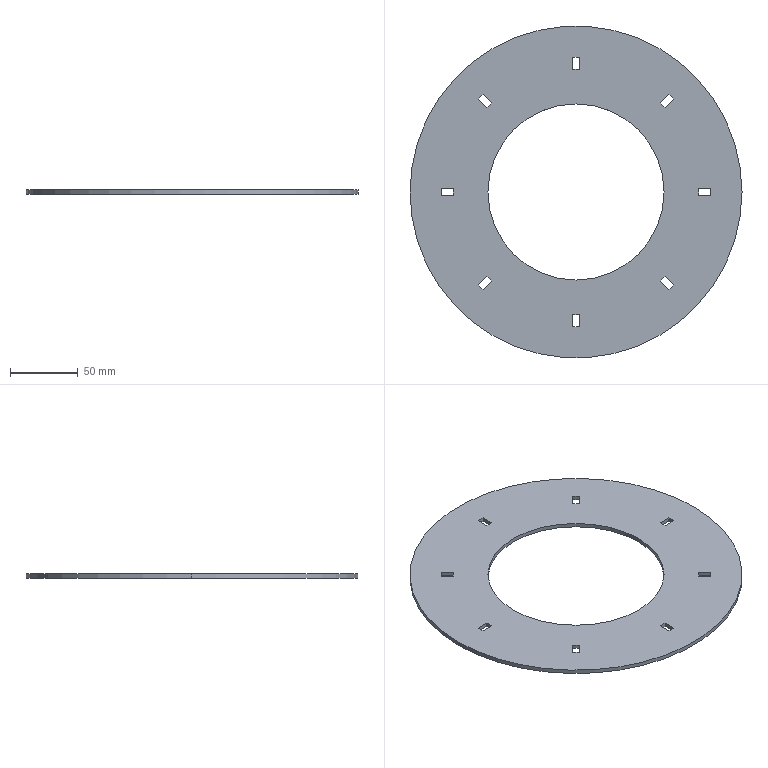Part | SolidWorks | features CirPattern 1, Extrusion 1, ICE 1 | 1 solid | 38 faces | box 245 x 245 x 3 mm | volume 100531 mm3 | plane 34 | cylinder 4 | commonest cylinder face diameters 130 x2 245 x2
STEP:
#1=CARTESIAN_POINT('',(-65.,0.,3.));
#2=VERTEX_POINT('',#1);
#3=CARTESIAN_POINT('',(65.,0.,3.));
#4=VERTEX_POINT('',#3);
#5=CARTESIAN_POINT('',(0.,0.,3.));
#6=DIRECTION('',(0.,0.,1.));
#7=DIRECTION('',(1.,0.,0.));
#8=AXIS2_PLACEMENT_3D('',#5,#6,#7);
#9=CIRCLE('',#8,65.);
#10=EDGE_CURVE('',#2,#4,#9,.T.);
#11=ORIENTED_EDGE('',*,*,#10,.T.);
#12=CARTESIAN_POINT('',(65.,0.,0.));
#13=VERTEX_POINT('',#12);
#14=CARTESIAN_POINT('',(65.,0.,3.));
#15=DIRECTION('',(0.,0.,-1.));
#16=VECTOR('',#15,1000.);
#17=LINE('',#14,#16);
#18=EDGE_CURVE('',#4,#13,#17,.T.);
#19=ORIENTED_EDGE('',*,*,#18,.T.);
#20=CARTESIAN_POINT('',(-65.,0.,0.));
#21=VERTEX_POINT('',#20);
#22=CARTESIAN_POINT('',(0.,0.,0.));
#23=DIRECTION('',(0.,0.,1.));
#24=DIRECTION('',(1.,0.,0.));
#25=AXIS2_PLACEMENT_3D('',#22,#23,#24);
#26=CIRCLE('',#25,65.);
#27=EDGE_CURVE('',#21,#13,#26,.T.);
#28=ORIENTED_EDGE('',*,*,#27,.F.);
#29=CARTESIAN_POINT('',(-65.,0.,3.));
#30=DIRECTION('',(0.,0.,-1.));
#31=VECTOR('',#30,1000.);
#32=LINE('',#29,#31);
#33=EDGE_CURVE('',#2,#21,#32,.T.);
#34=ORIENTED_EDGE('',*,*,#33,.F.);
#35=EDGE_LOOP('',(#11,#19,#28,#34));
#36=FACE_OUTER_BOUND('',#35,.T.);
#37=CARTESIAN_POINT('',(0.,0.,3.));
#38=DIRECTION('',(0.,0.,-1.));
#39=DIRECTION('',(-1.,0.,0.));
#40=AXIS2_PLACEMENT_3D('',#37,#38,#39);
#41=CYLINDRICAL_SURFACE('',#40,65.);
#42=ADVANCED_FACE('',(#36),#41,.F.);
#43=CARTESIAN_POINT('',(122.5,0.,3.));
#44=VERTEX_POINT('',#43);
#45=CARTESIAN_POINT('',(-122.5,0.,3.));
#46=VERTEX_POINT('',#45);
#47=CARTESIAN_POINT('',(0.,0.,3.));
#48=DIRECTION('',(0.,0.,1.));
#49=DIRECTION('',(1.,0.,0.));
#50=AXIS2_PLACEMENT_3D('',#47,#48,#49);
#51=CIRCLE('',#50,122.5);
#52=EDGE_CURVE('',#44,#46,#51,.T.);
#53=ORIENTED_EDGE('',*,*,#52,.F.);
#54=CARTESIAN_POINT('',(122.5,0.,0.));
#55=VERTEX_POINT('',#54);
#56=CARTESIAN_POINT('',(122.5,0.,3.));
#57=DIRECTION('',(0.,0.,-1.));
#58=VECTOR('',#57,1000.);
#59=LINE('',#56,#58);
#60=EDGE_CURVE('',#44,#55,#59,.T.);
#61=ORIENTED_EDGE('',*,*,#60,.T.);
#62=CARTESIAN_POINT('',(-122.5,0.,0.));
#63=VERTEX_POINT('',#62);
#64=CARTESIAN_POINT('',(0.,0.,0.));
#65=DIRECTION('',(0.,0.,1.));
#66=DIRECTION('',(1.,0.,0.));
#67=AXIS2_PLACEMENT_3D('',#64,#65,#66);
#68=CIRCLE('',#67,122.5);
#69=EDGE_CURVE('',#55,#63,#68,.T.);
#70=ORIENTED_EDGE('',*,*,#69,.T.);
#71=CARTESIAN_POINT('',(-122.5,0.,3.));
#72=DIRECTION('',(0.,0.,-1.));
#73=VECTOR('',#72,1000.);
#74=LINE('',#71,#73);
#75=EDGE_CURVE('',#46,#63,#74,.T.);
#76=ORIENTED_EDGE('',*,*,#75,.F.);
#77=EDGE_LOOP('',(#53,#61,#70,#76));
#78=FACE_OUTER_BOUND('',#77,.T.);
#79=CARTESIAN_POINT('',(0.,0.,3.));
#80=DIRECTION('',(0.,0.,-1.));
#81=DIRECTION('',(-1.,0.,0.));
#82=AXIS2_PLACEMENT_3D('',#79,#80,#81);
#83=CYLINDRICAL_SURFACE('',#82,122.5);
#84=ADVANCED_FACE('',(#78),#83,.T.);
#85=CARTESIAN_POINT('',(99.5,2.5,3.));
#86=VERTEX_POINT('',#85);
#87=CARTESIAN_POINT('',(90.5,2.5,3.));
#88=VERTEX_POINT('',#87);
#89=CARTESIAN_POINT('',(90.5,2.5,3.));
#90=DIRECTION('',(-1.,0.,0.));
#91=VECTOR('',#90,1000.);
#92=LINE('',#89,#91);
#93=EDGE_CURVE('',#86,#88,#92,.T.);
#94=ORIENTED_EDGE('',*,*,#93,.F.);
#95=CARTESIAN_POINT('',(99.5,-2.5,3.));
#96=VERTEX_POINT('',#95);
#97=CARTESIAN_POINT('',(99.5,-2.5,3.));
#98=DIRECTION('',(0.,1.,0.));
#99=VECTOR('',#98,1000.);
#100=LINE('',#97,#99);
#101=EDGE_CURVE('',#96,#86,#100,.T.);
#102=ORIENTED_EDGE('',*,*,#101,.F.);
#103=CARTESIAN_POINT('',(90.5,-2.5,3.));
#104=VERTEX_POINT('',#103);
#105=CARTESIAN_POINT('',(90.5,-2.5,3.));
#106=DIRECTION('',(1.,0.,0.));
#107=VECTOR('',#106,1000.);
#108=LINE('',#105,#107);
#109=EDGE_CURVE('',#104,#96,#108,.T.);
#110=ORIENTED_EDGE('',*,*,#109,.F.);
#111=CARTESIAN_POINT('',(90.5,-2.5,3.));
#112=DIRECTION('',(0.,-1.,0.));
#113=VECTOR('',#112,1000.);
#114=LINE('',#111,#113);
#115=EDGE_CURVE('',#88,#104,#114,.T.);
#116=ORIENTED_EDGE('',*,*,#115,.F.);
#117=EDGE_LOOP('',(#94,#102,#110,#116));
#118=FACE_BOUND('',#117,.T.);
#119=CARTESIAN_POINT('',(72.125,-68.589,3.));
#120=VERTEX_POINT('',#119);
#121=CARTESIAN_POINT('',(65.761,-62.225,3.));
#122=VERTEX_POINT('',#121);
#123=CARTESIAN_POINT('',(65.761,-62.225,3.));
#124=DIRECTION('',(-0.7071,0.7071,0.));
#125=VECTOR('',#124,1000.);
#126=LINE('',#123,#125);
#127=EDGE_CURVE('',#120,#122,#126,.T.);
#128=ORIENTED_EDGE('',*,*,#127,.F.);
#129=CARTESIAN_POINT('',(68.589,-72.125,3.));
#130=VERTEX_POINT('',#129);
#131=CARTESIAN_POINT('',(68.589,-72.125,3.));
#132=DIRECTION('',(0.7071,0.7071,0.));
#133=VECTOR('',#132,1000.);
#134=LINE('',#131,#133);
#135=EDGE_CURVE('',#130,#120,#134,.T.);
#136=ORIENTED_EDGE('',*,*,#135,.F.);
#137=CARTESIAN_POINT('',(62.225,-65.761,3.));
#138=VERTEX_POINT('',#137);
#139=CARTESIAN_POINT('',(62.225,-65.761,3.));
#140=DIRECTION('',(0.7071,-0.7071,0.));
#141=VECTOR('',#140,1000.);
#142=LINE('',#139,#141);
#143=EDGE_CURVE('',#138,#130,#142,.T.);
#144=ORIENTED_EDGE('',*,*,#143,.F.);
#145=CARTESIAN_POINT('',(62.225,-65.761,3.));
#146=DIRECTION('',(-0.7071,-0.7071,0.));
#147=VECTOR('',#146,1000.);
#148=LINE('',#145,#147);
#149=EDGE_CURVE('',#122,#138,#148,.T.);
#150=ORIENTED_EDGE('',*,*,#149,.F.);
#151=EDGE_LOOP('',(#128,#136,#144,#150));
#152=FACE_BOUND('',#151,.T.);
#153=CARTESIAN_POINT('',(2.5,-99.5,3.));
#154=VERTEX_POINT('',#153);
#155=CARTESIAN_POINT('',(2.5,-90.5,3.));
#156=VERTEX_POINT('',#155);
#157=CARTESIAN_POINT('',(2.5,-90.5,3.));
#158=DIRECTION('',(0.,1.,0.));
#159=VECTOR('',#158,1000.);
#160=LINE('',#157,#159);
#161=EDGE_CURVE('',#154,#156,#160,.T.);
#162=ORIENTED_EDGE('',*,*,#161,.F.);
#163=CARTESIAN_POINT('',(-2.5,-99.5,3.));
#164=VERTEX_POINT('',#163);
#165=CARTESIAN_POINT('',(-2.5,-99.5,3.));
#166=DIRECTION('',(1.,0.,0.));
#167=VECTOR('',#166,1000.);
#168=LINE('',#165,#167);
#169=EDGE_CURVE('',#164,#154,#168,.T.);
#170=ORIENTED_EDGE('',*,*,#169,.F.);
#171=CARTESIAN_POINT('',(-2.5,-90.5,3.));
#172=VERTEX_POINT('',#171);
#173=CARTESIAN_POINT('',(-2.5,-90.5,3.));
#174=DIRECTION('',(0.,-1.,0.));
#175=VECTOR('',#174,1000.);
#176=LINE('',#173,#175);
#177=EDGE_CURVE('',#172,#164,#176,.T.);
#178=ORIENTED_EDGE('',*,*,#177,.F.);
#179=CARTESIAN_POINT('',(-2.5,-90.5,3.));
#180=DIRECTION('',(-1.,0.,0.));
#181=VECTOR('',#180,1000.);
#182=LINE('',#179,#181);
#183=EDGE_CURVE('',#156,#172,#182,.T.);
#184=ORIENTED_EDGE('',*,*,#183,.F.);
#185=EDGE_LOOP('',(#162,#170,#178,#184));
#186=FACE_BOUND('',#185,.T.);
#187=CARTESIAN_POINT('',(-68.589,-72.125,3.));
#188=VERTEX_POINT('',#187);
#189=CARTESIAN_POINT('',(-62.225,-65.761,3.));
#190=VERTEX_POINT('',#189);
#191=CARTESIAN_POINT('',(-62.225,-65.761,3.));
#192=DIRECTION('',(0.7071,0.7071,0.));
#193=VECTOR('',#192,1000.);
#194=LINE('',#191,#193);
#195=EDGE_CURVE('',#188,#190,#194,.T.);
#196=ORIENTED_EDGE('',*,*,#195,.F.);
#197=CARTESIAN_POINT('',(-72.125,-68.589,3.));
#198=VERTEX_POINT('',#197);
#199=CARTESIAN_POINT('',(-72.125,-68.589,3.));
#200=DIRECTION('',(0.7071,-0.7071,0.));
#201=VECTOR('',#200,1000.);
#202=LINE('',#199,#201);
#203=EDGE_CURVE('',#198,#188,#202,.T.);
#204=ORIENTED_EDGE('',*,*,#203,.F.);
#205=CARTESIAN_POINT('',(-65.761,-62.225,3.));
#206=VERTEX_POINT('',#205);
#207=CARTESIAN_POINT('',(-65.761,-62.225,3.));
#208=DIRECTION('',(-0.7071,-0.7071,0.));
#209=VECTOR('',#208,1000.);
#210=LINE('',#207,#209);
#211=EDGE_CURVE('',#206,#198,#210,.T.);
#212=ORIENTED_EDGE('',*,*,#211,.F.);
#213=CARTESIAN_POINT('',(-65.761,-62.225,3.));
#214=DIRECTION('',(-0.7071,0.7071,0.));
#215=VECTOR('',#214,1000.);
#216=LINE('',#213,#215);
#217=EDGE_CURVE('',#190,#206,#216,.T.);
#218=ORIENTED_EDGE('',*,*,#217,.F.);
#219=EDGE_LOOP('',(#196,#204,#212,#218));
#220=FACE_BOUND('',#219,.T.);
#221=CARTESIAN_POINT('',(-99.5,-2.5,3.));
#222=VERTEX_POINT('',#221);
#223=CARTESIAN_POINT('',(-90.5,-2.5,3.));
#224=VERTEX_POINT('',#223);
#225=CARTESIAN_POINT('',(-90.5,-2.5,3.));
#226=DIRECTION('',(1.,0.,0.));
#227=VECTOR('',#226,1000.);
#228=LINE('',#225,#227);
#229=EDGE_CURVE('',#222,#224,#228,.T.);
#230=ORIENTED_EDGE('',*,*,#229,.F.);
#231=CARTESIAN_POINT('',(-99.5,2.5,3.));
#232=VERTEX_POINT('',#231);
#233=CARTESIAN_POINT('',(-99.5,2.5,3.));
#234=DIRECTION('',(0.,-1.,0.));
#235=VECTOR('',#234,1000.);
#236=LINE('',#233,#235);
#237=EDGE_CURVE('',#232,#222,#236,.T.);
#238=ORIENTED_EDGE('',*,*,#237,.F.);
#239=CARTESIAN_POINT('',(-90.5,2.5,3.));
#240=VERTEX_POINT('',#239);
#241=CARTESIAN_POINT('',(-90.5,2.5,3.));
#242=DIRECTION('',(-1.,0.,0.));
#243=VECTOR('',#242,1000.);
#244=LINE('',#241,#243);
#245=EDGE_CURVE('',#240,#232,#244,.T.);
#246=ORIENTED_EDGE('',*,*,#245,.F.);
#247=CARTESIAN_POINT('',(-90.5,2.5,3.));
#248=DIRECTION('',(0.,1.,0.));
#249=VECTOR('',#248,1000.);
#250=LINE('',#247,#249);
#251=EDGE_CURVE('',#224,#240,#250,.T.);
#252=ORIENTED_EDGE('',*,*,#251,.F.);
#253=EDGE_LOOP('',(#230,#238,#246,#252));
#254=FACE_BOUND('',#253,.T.);
#255=CARTESIAN_POINT('',(-72.125,68.589,3.));
#256=VERTEX_POINT('',#255);
#257=CARTESIAN_POINT('',(-65.761,62.225,3.));
#258=VERTEX_POINT('',#257);
#259=CARTESIAN_POINT('',(-65.761,62.225,3.));
#260=DIRECTION('',(0.7071,-0.7071,0.));
#261=VECTOR('',#260,1000.);
#262=LINE('',#259,#261);
#263=EDGE_CURVE('',#256,#258,#262,.T.);
#264=ORIENTED_EDGE('',*,*,#263,.F.);
#265=CARTESIAN_POINT('',(-68.589,72.125,3.));
#266=VERTEX_POINT('',#265);
#267=CARTESIAN_POINT('',(-68.589,72.125,3.));
#268=DIRECTION('',(-0.7071,-0.7071,0.));
#269=VECTOR('',#268,1000.);
#270=LINE('',#267,#269);
#271=EDGE_CURVE('',#266,#256,#270,.T.);
#272=ORIENTED_EDGE('',*,*,#271,.F.);
#273=CARTESIAN_POINT('',(-62.225,65.761,3.));
#274=VERTEX_POINT('',#273);
#275=CARTESIAN_POINT('',(-62.225,65.761,3.));
#276=DIRECTION('',(-0.7071,0.7071,0.));
#277=VECTOR('',#276,1000.);
#278=LINE('',#275,#277);
#279=EDGE_CURVE('',#274,#266,#278,.T.);
#280=ORIENTED_EDGE('',*,*,#279,.F.);
#281=CARTESIAN_POINT('',(-62.225,65.761,3.));
#282=DIRECTION('',(0.7071,0.7071,0.));
#283=VECTOR('',#282,1000.);
#284=LINE('',#281,#283);
#285=EDGE_CURVE('',#258,#274,#284,.T.);
#286=ORIENTED_EDGE('',*,*,#285,.F.);
#287=EDGE_LOOP('',(#264,#272,#280,#286));
#288=FACE_BOUND('',#287,.T.);
#289=CARTESIAN_POINT('',(68.589,72.125,3.));
#290=VERTEX_POINT('',#289);
#291=CARTESIAN_POINT('',(62.225,65.761,3.));
#292=VERTEX_POINT('',#291);
#293=CARTESIAN_POINT('',(62.225,65.761,3.));
#294=DIRECTION('',(-0.7071,-0.7071,0.));
#295=VECTOR('',#294,1000.);
#296=LINE('',#293,#295);
#297=EDGE_CURVE('',#290,#292,#296,.T.);
#298=ORIENTED_EDGE('',*,*,#297,.F.);
#299=CARTESIAN_POINT('',(72.125,68.589,3.));
#300=VERTEX_POINT('',#299);
#301=CARTESIAN_POINT('',(72.125,68.589,3.));
#302=DIRECTION('',(-0.7071,0.7071,0.));
#303=VECTOR('',#302,1000.);
#304=LINE('',#301,#303);
#305=EDGE_CURVE('',#300,#290,#304,.T.);
#306=ORIENTED_EDGE('',*,*,#305,.F.);
#307=CARTESIAN_POINT('',(65.761,62.225,3.));
#308=VERTEX_POINT('',#307);
#309=CARTESIAN_POINT('',(65.761,62.225,3.));
#310=DIRECTION('',(0.7071,0.7071,0.));
#311=VECTOR('',#310,1000.);
#312=LINE('',#309,#311);
#313=EDGE_CURVE('',#308,#300,#312,.T.);
#314=ORIENTED_EDGE('',*,*,#313,.F.);
#315=CARTESIAN_POINT('',(65.761,62.225,3.));
#316=DIRECTION('',(0.7071,-0.7071,0.));
#317=VECTOR('',#316,1000.);
#318=LINE('',#315,#317);
#319=EDGE_CURVE('',#292,#308,#318,.T.);
#320=ORIENTED_EDGE('',*,*,#319,.F.);
#321=EDGE_LOOP('',(#298,#306,#314,#320));
#322=FACE_BOUND('',#321,.T.);
#323=CARTESIAN_POINT('',(-2.5,99.5,3.));
#324=VERTEX_POINT('',#323);
#325=CARTESIAN_POINT('',(-2.5,90.5,3.));
#326=VERTEX_POINT('',#325);
#327=CARTESIAN_POINT('',(-2.5,90.5,3.));
#328=DIRECTION('',(0.,-1.,0.));
#329=VECTOR('',#328,1000.);
#330=LINE('',#327,#329);
#331=EDGE_CURVE('',#324,#326,#330,.T.);
#332=ORIENTED_EDGE('',*,*,#331,.F.);
#333=CARTESIAN_POINT('',(2.5,99.5,3.));
#334=VERTEX_POINT('',#333);
#335=CARTESIAN_POINT('',(2.5,99.5,3.));
#336=DIRECTION('',(-1.,0.,0.));
#337=VECTOR('',#336,1000.);
#338=LINE('',#335,#337);
#339=EDGE_CURVE('',#334,#324,#338,.T.);
#340=ORIENTED_EDGE('',*,*,#339,.F.);
#341=CARTESIAN_POINT('',(2.5,90.5,3.));
#342=VERTEX_POINT('',#341);
#343=CARTESIAN_POINT('',(2.5,90.5,3.));
#344=DIRECTION('',(0.,1.,0.));
#345=VECTOR('',#344,1000.);
#346=LINE('',#343,#345);
#347=EDGE_CURVE('',#342,#334,#346,.T.);
#348=ORIENTED_EDGE('',*,*,#347,.F.);
#349=CARTESIAN_POINT('',(2.5,90.5,3.));
#350=DIRECTION('',(1.,0.,0.));
#351=VECTOR('',#350,1000.);
#352=LINE('',#349,#351);
#353=EDGE_CURVE('',#326,#342,#352,.T.);
#354=ORIENTED_EDGE('',*,*,#353,.F.);
#355=EDGE_LOOP('',(#332,#340,#348,#354));
#356=FACE_BOUND('',#355,.T.);
#357=CARTESIAN_POINT('',(0.,0.,3.));
#358=DIRECTION('',(0.,0.,1.));
#359=DIRECTION('',(1.,0.,0.));
#360=AXIS2_PLACEMENT_3D('',#357,#358,#359);
#361=CIRCLE('',#360,122.5);
#362=EDGE_CURVE('',#46,#44,#361,.T.);
#363=ORIENTED_EDGE('',*,*,#362,.T.);
#364=ORIENTED_EDGE('',*,*,#52,.T.);
#365=EDGE_LOOP('',(#363,#364));
#366=FACE_OUTER_BOUND('',#365,.T.);
#367=ORIENTED_EDGE('',*,*,#10,.F.);
#368=CARTESIAN_POINT('',(0.,0.,3.));
#369=DIRECTION('',(0.,0.,1.));
#370=DIRECTION('',(1.,0.,0.));
#371=AXIS2_PLACEMENT_3D('',#368,#369,#370);
#372=CIRCLE('',#371,65.);
#373=EDGE_CURVE('',#4,#2,#372,.T.);
#374=ORIENTED_EDGE('',*,*,#373,.F.);
#375=EDGE_LOOP('',(#367,#374));
#376=FACE_BOUND('',#375,.T.);
#377=CARTESIAN_POINT('',(0.,0.,3.));
#378=DIRECTION('',(0.,0.,1.));
#379=DIRECTION('',(1.,0.,0.));
#380=AXIS2_PLACEMENT_3D('',#377,#378,#379);
#381=PLANE('',#380);
#382=ADVANCED_FACE('',(#118,#152,#186,#220,#254,#288,#322,#356,#366,#376),#381,.T.);
#383=CARTESIAN_POINT('',(99.5,-2.5,0.));
#384=VERTEX_POINT('',#383);
#385=CARTESIAN_POINT('',(99.5,2.5,0.));
#386=VERTEX_POINT('',#385);
#387=CARTESIAN_POINT('',(99.5,0.,0.));
#388=DIRECTION('',(0.,1.,0.));
#389=VECTOR('',#388,1000.);
#390=LINE('',#387,#389);
#391=EDGE_CURVE('',#384,#386,#390,.T.);
#392=ORIENTED_EDGE('',*,*,#391,.T.);
#393=CARTESIAN_POINT('',(90.5,2.5,0.));
#394=VERTEX_POINT('',#393);
#395=CARTESIAN_POINT('',(0.,2.5,0.));
#396=DIRECTION('',(-1.,0.,0.));
#397=VECTOR('',#396,1000.);
#398=LINE('',#395,#397);
#399=EDGE_CURVE('',#386,#394,#398,.T.);
#400=ORIENTED_EDGE('',*,*,#399,.T.);
#401=CARTESIAN_POINT('',(90.5,-2.5,0.));
#402=VERTEX_POINT('',#401);
#403=CARTESIAN_POINT('',(90.5,0.,0.));
#404=DIRECTION('',(0.,-1.,0.));
#405=VECTOR('',#404,1000.);
#406=LINE('',#403,#405);
#407=EDGE_CURVE('',#394,#402,#406,.T.);
#408=ORIENTED_EDGE('',*,*,#407,.T.);
#409=CARTESIAN_POINT('',(0.,-2.5,0.));
#410=DIRECTION('',(1.,0.,0.));
#411=VECTOR('',#410,1000.);
#412=LINE('',#409,#411);
#413=EDGE_CURVE('',#402,#384,#412,.T.);
#414=ORIENTED_EDGE('',*,*,#413,.T.);
#415=EDGE_LOOP('',(#392,#400,#408,#414));
#416=FACE_BOUND('',#415,.T.);
#417=CARTESIAN_POINT('',(68.589,-72.125,0.));
#418=VERTEX_POINT('',#417);
#419=CARTESIAN_POINT('',(72.125,-68.589,0.));
#420=VERTEX_POINT('',#419);
#421=CARTESIAN_POINT('',(70.357,-70.357,0.));
#422=DIRECTION('',(0.7071,0.7071,0.));
#423=VECTOR('',#422,1000.);
#424=LINE('',#421,#423);
#425=EDGE_CURVE('',#418,#420,#424,.T.);
#426=ORIENTED_EDGE('',*,*,#425,.T.);
#427=CARTESIAN_POINT('',(65.761,-62.225,0.));
#428=VERTEX_POINT('',#427);
#429=CARTESIAN_POINT('',(1.768,1.768,0.));
#430=DIRECTION('',(-0.7071,0.7071,0.));
#431=VECTOR('',#430,1000.);
#432=LINE('',#429,#431);
#433=EDGE_CURVE('',#420,#428,#432,.T.);
#434=ORIENTED_EDGE('',*,*,#433,.T.);
#435=CARTESIAN_POINT('',(62.225,-65.761,0.));
#436=VERTEX_POINT('',#435);
#437=CARTESIAN_POINT('',(63.993,-63.993,0.));
#438=DIRECTION('',(-0.7071,-0.7071,0.));
#439=VECTOR('',#438,1000.);
#440=LINE('',#437,#439);
#441=EDGE_CURVE('',#428,#436,#440,.T.);
#442=ORIENTED_EDGE('',*,*,#441,.T.);
#443=CARTESIAN_POINT('',(-1.768,-1.768,0.));
#444=DIRECTION('',(0.7071,-0.7071,0.));
#445=VECTOR('',#444,1000.);
#446=LINE('',#443,#445);
#447=EDGE_CURVE('',#436,#418,#446,.T.);
#448=ORIENTED_EDGE('',*,*,#447,.T.);
#449=EDGE_LOOP('',(#426,#434,#442,#448));
#450=FACE_BOUND('',#449,.T.);
#451=CARTESIAN_POINT('',(-2.5,-99.5,0.));
#452=VERTEX_POINT('',#451);
#453=CARTESIAN_POINT('',(2.5,-99.5,0.));
#454=VERTEX_POINT('',#453);
#455=CARTESIAN_POINT('',(0.,-99.5,0.));
#456=DIRECTION('',(1.,0.,0.));
#457=VECTOR('',#456,1000.);
#458=LINE('',#455,#457);
#459=EDGE_CURVE('',#452,#454,#458,.T.);
#460=ORIENTED_EDGE('',*,*,#459,.T.);
#461=CARTESIAN_POINT('',(2.5,-90.5,0.));
#462=VERTEX_POINT('',#461);
#463=CARTESIAN_POINT('',(2.5,0.,0.));
#464=DIRECTION('',(0.,1.,0.));
#465=VECTOR('',#464,1000.);
#466=LINE('',#463,#465);
#467=EDGE_CURVE('',#454,#462,#466,.T.);
#468=ORIENTED_EDGE('',*,*,#467,.T.);
#469=CARTESIAN_POINT('',(-2.5,-90.5,0.));
#470=VERTEX_POINT('',#469);
#471=CARTESIAN_POINT('',(0.,-90.5,0.));
#472=DIRECTION('',(-1.,0.,0.));
#473=VECTOR('',#472,1000.);
#474=LINE('',#471,#473);
#475=EDGE_CURVE('',#462,#470,#474,.T.);
#476=ORIENTED_EDGE('',*,*,#475,.T.);
#477=CARTESIAN_POINT('',(-2.5,0.,0.));
#478=DIRECTION('',(0.,-1.,0.));
#479=VECTOR('',#478,1000.);
#480=LINE('',#477,#479);
#481=EDGE_CURVE('',#470,#452,#480,.T.);
#482=ORIENTED_EDGE('',*,*,#481,.T.);
#483=EDGE_LOOP('',(#460,#468,#476,#482));
#484=FACE_BOUND('',#483,.T.);
#485=CARTESIAN_POINT('',(-72.125,-68.589,0.));
#486=VERTEX_POINT('',#485);
#487=CARTESIAN_POINT('',(-68.589,-72.125,0.));
#488=VERTEX_POINT('',#487);
#489=CARTESIAN_POINT('',(-70.357,-70.357,0.));
#490=DIRECTION('',(0.7071,-0.7071,0.));
#491=VECTOR('',#490,1000.);
#492=LINE('',#489,#491);
#493=EDGE_CURVE('',#486,#488,#492,.T.);
#494=ORIENTED_EDGE('',*,*,#493,.T.);
#495=CARTESIAN_POINT('',(-62.225,-65.761,0.));
#496=VERTEX_POINT('',#495);
#497=CARTESIAN_POINT('',(1.768,-1.768,0.));
#498=DIRECTION('',(0.7071,0.7071,0.));
#499=VECTOR('',#498,1000.);
#500=LINE('',#497,#499);
#501=EDGE_CURVE('',#488,#496,#500,.T.);
#502=ORIENTED_EDGE('',*,*,#501,.T.);
#503=CARTESIAN_POINT('',(-65.761,-62.225,0.));
#504=VERTEX_POINT('',#503);
#505=CARTESIAN_POINT('',(-63.993,-63.993,0.));
#506=DIRECTION('',(-0.7071,0.7071,0.));
#507=VECTOR('',#506,1000.);
#508=LINE('',#505,#507);
#509=EDGE_CURVE('',#496,#504,#508,.T.);
#510=ORIENTED_EDGE('',*,*,#509,.T.);
#511=CARTESIAN_POINT('',(-1.768,1.768,0.));
#512=DIRECTION('',(-0.7071,-0.7071,0.));
#513=VECTOR('',#512,1000.);
#514=LINE('',#511,#513);
#515=EDGE_CURVE('',#504,#486,#514,.T.);
#516=ORIENTED_EDGE('',*,*,#515,.T.);
#517=EDGE_LOOP('',(#494,#502,#510,#516));
#518=FACE_BOUND('',#517,.T.);
#519=CARTESIAN_POINT('',(-99.5,2.5,0.));
#520=VERTEX_POINT('',#519);
#521=CARTESIAN_POINT('',(-99.5,-2.5,0.));
#522=VERTEX_POINT('',#521);
#523=CARTESIAN_POINT('',(-99.5,0.,0.));
#524=DIRECTION('',(0.,-1.,0.));
#525=VECTOR('',#524,1000.);
#526=LINE('',#523,#525);
#527=EDGE_CURVE('',#520,#522,#526,.T.);
#528=ORIENTED_EDGE('',*,*,#527,.T.);
#529=CARTESIAN_POINT('',(-90.5,-2.5,0.));
#530=VERTEX_POINT('',#529);
#531=CARTESIAN_POINT('',(0.,-2.5,0.));
#532=DIRECTION('',(1.,0.,0.));
#533=VECTOR('',#532,1000.);
#534=LINE('',#531,#533);
#535=EDGE_CURVE('',#522,#530,#534,.T.);
#536=ORIENTED_EDGE('',*,*,#535,.T.);
#537=CARTESIAN_POINT('',(-90.5,2.5,0.));
#538=VERTEX_POINT('',#537);
#539=CARTESIAN_POINT('',(-90.5,0.,0.));
#540=DIRECTION('',(0.,1.,0.));
#541=VECTOR('',#540,1000.);
#542=LINE('',#539,#541);
#543=EDGE_CURVE('',#530,#538,#542,.T.);
#544=ORIENTED_EDGE('',*,*,#543,.T.);
#545=CARTESIAN_POINT('',(0.,2.5,0.));
#546=DIRECTION('',(-1.,0.,0.));
#547=VECTOR('',#546,1000.);
#548=LINE('',#545,#547);
#549=EDGE_CURVE('',#538,#520,#548,.T.);
#550=ORIENTED_EDGE('',*,*,#549,.T.);
#551=EDGE_LOOP('',(#528,#536,#544,#550));
#552=FACE_BOUND('',#551,.T.);
#553=CARTESIAN_POINT('',(-68.589,72.125,0.));
#554=VERTEX_POINT('',#553);
#555=CARTESIAN_POINT('',(-72.125,68.589,0.));
#556=VERTEX_POINT('',#555);
#557=CARTESIAN_POINT('',(-70.357,70.357,0.));
#558=DIRECTION('',(-0.7071,-0.7071,0.));
#559=VECTOR('',#558,1000.);
#560=LINE('',#557,#559);
#561=EDGE_CURVE('',#554,#556,#560,.T.);
#562=ORIENTED_EDGE('',*,*,#561,.T.);
#563=CARTESIAN_POINT('',(-65.761,62.225,0.));
#564=VERTEX_POINT('',#563);
#565=CARTESIAN_POINT('',(-1.768,-1.768,0.));
#566=DIRECTION('',(0.7071,-0.7071,0.));
#567=VECTOR('',#566,1000.);
#568=LINE('',#565,#567);
#569=EDGE_CURVE('',#556,#564,#568,.T.);
#570=ORIENTED_EDGE('',*,*,#569,.T.);
#571=CARTESIAN_POINT('',(-62.225,65.761,0.));
#572=VERTEX_POINT('',#571);
#573=CARTESIAN_POINT('',(-63.993,63.993,0.));
#574=DIRECTION('',(0.7071,0.7071,0.));
#575=VECTOR('',#574,1000.);
#576=LINE('',#573,#575);
#577=EDGE_CURVE('',#564,#572,#576,.T.);
#578=ORIENTED_EDGE('',*,*,#577,.T.);
#579=CARTESIAN_POINT('',(1.768,1.768,0.));
#580=DIRECTION('',(-0.7071,0.7071,0.));
#581=VECTOR('',#580,1000.);
#582=LINE('',#579,#581);
#583=EDGE_CURVE('',#572,#554,#582,.T.);
#584=ORIENTED_EDGE('',*,*,#583,.T.);
#585=EDGE_LOOP('',(#562,#570,#578,#584));
#586=FACE_BOUND('',#585,.T.);
#587=CARTESIAN_POINT('',(72.125,68.589,0.));
#588=VERTEX_POINT('',#587);
#589=CARTESIAN_POINT('',(68.589,72.125,0.));
#590=VERTEX_POINT('',#589);
#591=CARTESIAN_POINT('',(70.357,70.357,0.));
#592=DIRECTION('',(-0.7071,0.7071,0.));
#593=VECTOR('',#592,1000.);
#594=LINE('',#591,#593);
#595=EDGE_CURVE('',#588,#590,#594,.T.);
#596=ORIENTED_EDGE('',*,*,#595,.T.);
#597=CARTESIAN_POINT('',(62.225,65.761,0.));
#598=VERTEX_POINT('',#597);
#599=CARTESIAN_POINT('',(-1.768,1.768,0.));
#600=DIRECTION('',(-0.7071,-0.7071,0.));
#601=VECTOR('',#600,1000.);
#602=LINE('',#599,#601);
#603=EDGE_CURVE('',#590,#598,#602,.T.);
#604=ORIENTED_EDGE('',*,*,#603,.T.);
#605=CARTESIAN_POINT('',(65.761,62.225,0.));
#606=VERTEX_POINT('',#605);
#607=CARTESIAN_POINT('',(63.993,63.993,0.));
#608=DIRECTION('',(0.7071,-0.7071,0.));
#609=VECTOR('',#608,1000.);
#610=LINE('',#607,#609);
#611=EDGE_CURVE('',#598,#606,#610,.T.);
#612=ORIENTED_EDGE('',*,*,#611,.T.);
#613=CARTESIAN_POINT('',(1.768,-1.768,0.));
#614=DIRECTION('',(0.7071,0.7071,0.));
#615=VECTOR('',#614,1000.);
#616=LINE('',#613,#615);
#617=EDGE_CURVE('',#606,#588,#616,.T.);
#618=ORIENTED_EDGE('',*,*,#617,.T.);
#619=EDGE_LOOP('',(#596,#604,#612,#618));
#620=FACE_BOUND('',#619,.T.);
#621=CARTESIAN_POINT('',(2.5,99.5,0.));
#622=VERTEX_POINT('',#621);
#623=CARTESIAN_POINT('',(-2.5,99.5,0.));
#624=VERTEX_POINT('',#623);
#625=CARTESIAN_POINT('',(0.,99.5,0.));
#626=DIRECTION('',(-1.,0.,0.));
#627=VECTOR('',#626,1000.);
#628=LINE('',#625,#627);
#629=EDGE_CURVE('',#622,#624,#628,.T.);
#630=ORIENTED_EDGE('',*,*,#629,.T.);
#631=CARTESIAN_POINT('',(-2.5,90.5,0.));
#632=VERTEX_POINT('',#631);
#633=CARTESIAN_POINT('',(-2.5,0.,0.));
#634=DIRECTION('',(0.,-1.,0.));
#635=VECTOR('',#634,1000.);
#636=LINE('',#633,#635);
#637=EDGE_CURVE('',#624,#632,#636,.T.);
#638=ORIENTED_EDGE('',*,*,#637,.T.);
#639=CARTESIAN_POINT('',(2.5,90.5,0.));
#640=VERTEX_POINT('',#639);
#641=CARTESIAN_POINT('',(0.,90.5,0.));
#642=DIRECTION('',(1.,0.,0.));
#643=VECTOR('',#642,1000.);
#644=LINE('',#641,#643);
#645=EDGE_CURVE('',#632,#640,#644,.T.);
#646=ORIENTED_EDGE('',*,*,#645,.T.);
#647=CARTESIAN_POINT('',(2.5,0.,0.));
#648=DIRECTION('',(0.,1.,0.));
#649=VECTOR('',#648,1000.);
#650=LINE('',#647,#649);
#651=EDGE_CURVE('',#640,#622,#650,.T.);
#652=ORIENTED_EDGE('',*,*,#651,.T.);
#653=EDGE_LOOP('',(#630,#638,#646,#652));
#654=FACE_BOUND('',#653,.T.);
#655=CARTESIAN_POINT('',(0.,0.,0.));
#656=DIRECTION('',(0.,0.,1.));
#657=DIRECTION('',(1.,0.,0.));
#658=AXIS2_PLACEMENT_3D('',#655,#656,#657);
#659=CIRCLE('',#658,122.5);
#660=EDGE_CURVE('',#63,#55,#659,.T.);
#661=ORIENTED_EDGE('',*,*,#660,.F.);
#662=ORIENTED_EDGE('',*,*,#69,.F.);
#663=EDGE_LOOP('',(#661,#662));
#664=FACE_OUTER_BOUND('',#663,.T.);
#665=ORIENTED_EDGE('',*,*,#27,.T.);
#666=CARTESIAN_POINT('',(0.,0.,0.));
#667=DIRECTION('',(0.,0.,1.));
#668=DIRECTION('',(1.,0.,0.));
#669=AXIS2_PLACEMENT_3D('',#666,#667,#668);
#670=CIRCLE('',#669,65.);
#671=EDGE_CURVE('',#13,#21,#670,.T.);
#672=ORIENTED_EDGE('',*,*,#671,.T.);
#673=EDGE_LOOP('',(#665,#672));
#674=FACE_BOUND('',#673,.T.);
#675=CARTESIAN_POINT('',(0.,0.,0.));
#676=DIRECTION('',(0.,0.,1.));
#677=DIRECTION('',(1.,0.,0.));
#678=AXIS2_PLACEMENT_3D('',#675,#676,#677);
#679=PLANE('',#678);
#680=ADVANCED_FACE('',(#416,#450,#484,#518,#552,#586,#620,#654,#664,#674),#679,.F.);
#681=ORIENTED_EDGE('',*,*,#60,.F.);
#682=ORIENTED_EDGE('',*,*,#362,.F.);
#683=ORIENTED_EDGE('',*,*,#75,.T.);
#684=ORIENTED_EDGE('',*,*,#660,.T.);
#685=EDGE_LOOP('',(#681,#682,#683,#684));
#686=FACE_OUTER_BOUND('',#685,.T.);
#687=CARTESIAN_POINT('',(0.,0.,3.));
#688=DIRECTION('',(0.,0.,-1.));
#689=DIRECTION('',(-1.,0.,0.));
#690=AXIS2_PLACEMENT_3D('',#687,#688,#689);
#691=CYLINDRICAL_SURFACE('',#690,122.5);
#692=ADVANCED_FACE('',(#686),#691,.T.);
#693=ORIENTED_EDGE('',*,*,#18,.F.);
#694=ORIENTED_EDGE('',*,*,#373,.T.);
#695=ORIENTED_EDGE('',*,*,#33,.T.);
#696=ORIENTED_EDGE('',*,*,#671,.F.);
#697=EDGE_LOOP('',(#693,#694,#695,#696));
#698=FACE_OUTER_BOUND('',#697,.T.);
#699=CARTESIAN_POINT('',(0.,0.,3.));
#700=DIRECTION('',(0.,0.,-1.));
#701=DIRECTION('',(-1.,0.,0.));
#702=AXIS2_PLACEMENT_3D('',#699,#700,#701);
#703=CYLINDRICAL_SURFACE('',#702,65.);
#704=ADVANCED_FACE('',(#698),#703,.F.);
#705=CARTESIAN_POINT('',(-2.5,99.5,-2.));
#706=DIRECTION('',(0.,0.,1.));
#707=VECTOR('',#706,1000.);
#708=LINE('',#705,#707);
#709=EDGE_CURVE('',#624,#324,#708,.T.);
#710=ORIENTED_EDGE('',*,*,#709,.T.);
#711=ORIENTED_EDGE('',*,*,#331,.T.);
#712=CARTESIAN_POINT('',(-2.5,90.5,-2.));
#713=DIRECTION('',(0.,0.,1.));
#714=VECTOR('',#713,1000.);
#715=LINE('',#712,#714);
#716=EDGE_CURVE('',#632,#326,#715,.T.);
#717=ORIENTED_EDGE('',*,*,#716,.F.);
#718=ORIENTED_EDGE('',*,*,#637,.F.);
#719=EDGE_LOOP('',(#710,#711,#717,#718));
#720=FACE_OUTER_BOUND('',#719,.T.);
#721=CARTESIAN_POINT('',(-2.5,90.5,-2.));
#722=DIRECTION('',(-1.,0.,0.));
#723=DIRECTION('',(0.,0.,1.));
#724=AXIS2_PLACEMENT_3D('',#721,#722,#723);
#725=PLANE('',#724);
#726=ADVANCED_FACE('',(#720),#725,.F.);
#727=CARTESIAN_POINT('',(2.5,99.5,-2.));
#728=DIRECTION('',(0.,0.,1.));
#729=VECTOR('',#728,1000.);
#730=LINE('',#727,#729);
#731=EDGE_CURVE('',#622,#334,#730,.T.);
#732=ORIENTED_EDGE('',*,*,#731,.T.);
#733=ORIENTED_EDGE('',*,*,#339,.T.);
#734=ORIENTED_EDGE('',*,*,#709,.F.);
#735=ORIENTED_EDGE('',*,*,#629,.F.);
#736=EDGE_LOOP('',(#732,#733,#734,#735));
#737=FACE_OUTER_BOUND('',#736,.T.);
#738=CARTESIAN_POINT('',(2.5,99.5,-2.));
#739=DIRECTION('',(0.,1.,0.));
#740=DIRECTION('',(0.,0.,1.));
#741=AXIS2_PLACEMENT_3D('',#738,#739,#740);
#742=PLANE('',#741);
#743=ADVANCED_FACE('',(#737),#742,.F.);
#744=CARTESIAN_POINT('',(2.5,90.5,-2.));
#745=DIRECTION('',(0.,0.,1.));
#746=VECTOR('',#745,1000.);
#747=LINE('',#744,#746);
#748=EDGE_CURVE('',#640,#342,#747,.T.);
#749=ORIENTED_EDGE('',*,*,#748,.T.);
#750=ORIENTED_EDGE('',*,*,#347,.T.);
#751=ORIENTED_EDGE('',*,*,#731,.F.);
#752=ORIENTED_EDGE('',*,*,#651,.F.);
#753=EDGE_LOOP('',(#749,#750,#751,#752));
#754=FACE_OUTER_BOUND('',#753,.T.);
#755=CARTESIAN_POINT('',(2.5,90.5,-2.));
#756=DIRECTION('',(1.,0.,0.));
#757=DIRECTION('',(0.,0.,-1.));
#758=AXIS2_PLACEMENT_3D('',#755,#756,#757);
#759=PLANE('',#758);
#760=ADVANCED_FACE('',(#754),#759,.F.);
#761=ORIENTED_EDGE('',*,*,#716,.T.);
#762=ORIENTED_EDGE('',*,*,#353,.T.);
#763=ORIENTED_EDGE('',*,*,#748,.F.);
#764=ORIENTED_EDGE('',*,*,#645,.F.);
#765=EDGE_LOOP('',(#761,#762,#763,#764));
#766=FACE_OUTER_BOUND('',#765,.T.);
#767=CARTESIAN_POINT('',(2.5,90.5,-2.));
#768=DIRECTION('',(0.,-1.,0.));
#769=DIRECTION('',(0.,0.,-1.));
#770=AXIS2_PLACEMENT_3D('',#767,#768,#769);
#771=PLANE('',#770);
#772=ADVANCED_FACE('',(#766),#771,.F.);
#773=CARTESIAN_POINT('',(68.589,72.125,-2.));
#774=DIRECTION('',(0.,0.,1.));
#775=VECTOR('',#774,1000.);
#776=LINE('',#773,#775);
#777=EDGE_CURVE('',#590,#290,#776,.T.);
#778=ORIENTED_EDGE('',*,*,#777,.T.);
#779=ORIENTED_EDGE('',*,*,#297,.T.);
#780=CARTESIAN_POINT('',(62.225,65.761,-2.));
#781=DIRECTION('',(0.,0.,1.));
#782=VECTOR('',#781,1000.);
#783=LINE('',#780,#782);
#784=EDGE_CURVE('',#598,#292,#783,.T.);
#785=ORIENTED_EDGE('',*,*,#784,.F.);
#786=ORIENTED_EDGE('',*,*,#603,.F.);
#787=EDGE_LOOP('',(#778,#779,#785,#786));
#788=FACE_OUTER_BOUND('',#787,.T.);
#789=CARTESIAN_POINT('',(62.225,65.761,-2.));
#790=DIRECTION('',(-0.7071,0.7071,0.));
#791=DIRECTION('',(-0.7071,-0.7071,0.));
#792=AXIS2_PLACEMENT_3D('',#789,#790,#791);
#793=PLANE('',#792);
#794=ADVANCED_FACE('',(#788),#793,.F.);
#795=CARTESIAN_POINT('',(72.125,68.589,-2.));
#796=DIRECTION('',(0.,0.,1.));
#797=VECTOR('',#796,1000.);
#798=LINE('',#795,#797);
#799=EDGE_CURVE('',#588,#300,#798,.T.);
#800=ORIENTED_EDGE('',*,*,#799,.T.);
#801=ORIENTED_EDGE('',*,*,#305,.T.);
#802=ORIENTED_EDGE('',*,*,#777,.F.);
#803=ORIENTED_EDGE('',*,*,#595,.F.);
#804=EDGE_LOOP('',(#800,#801,#802,#803));
#805=FACE_OUTER_BOUND('',#804,.T.);
#806=CARTESIAN_POINT('',(72.125,68.589,-2.));
#807=DIRECTION('',(0.7071,0.7071,0.));
#808=DIRECTION('',(-0.7071,0.7071,0.));
#809=AXIS2_PLACEMENT_3D('',#806,#807,#808);
#810=PLANE('',#809);
#811=ADVANCED_FACE('',(#805),#810,.F.);
#812=CARTESIAN_POINT('',(65.761,62.225,-2.));
#813=DIRECTION('',(0.,0.,1.));
#814=VECTOR('',#813,1000.);
#815=LINE('',#812,#814);
#816=EDGE_CURVE('',#606,#308,#815,.T.);
#817=ORIENTED_EDGE('',*,*,#816,.T.);
#818=ORIENTED_EDGE('',*,*,#313,.T.);
#819=ORIENTED_EDGE('',*,*,#799,.F.);
#820=ORIENTED_EDGE('',*,*,#617,.F.);
#821=EDGE_LOOP('',(#817,#818,#819,#820));
#822=FACE_OUTER_BOUND('',#821,.T.);
#823=CARTESIAN_POINT('',(65.761,62.225,-2.));
#824=DIRECTION('',(0.7071,-0.7071,0.));
#825=DIRECTION('',(0.7071,0.7071,0.));
#826=AXIS2_PLACEMENT_3D('',#823,#824,#825);
#827=PLANE('',#826);
#828=ADVANCED_FACE('',(#822),#827,.F.);
#829=ORIENTED_EDGE('',*,*,#784,.T.);
#830=ORIENTED_EDGE('',*,*,#319,.T.);
#831=ORIENTED_EDGE('',*,*,#816,.F.);
#832=ORIENTED_EDGE('',*,*,#611,.F.);
#833=EDGE_LOOP('',(#829,#830,#831,#832));
#834=FACE_OUTER_BOUND('',#833,.T.);
#835=CARTESIAN_POINT('',(65.761,62.225,-2.));
#836=DIRECTION('',(-0.7071,-0.7071,0.));
#837=DIRECTION('',(0.7071,-0.7071,0.));
#838=AXIS2_PLACEMENT_3D('',#835,#836,#837);
#839=PLANE('',#838);
#840=ADVANCED_FACE('',(#834),#839,.F.);
#841=CARTESIAN_POINT('',(-72.125,68.589,-2.));
#842=DIRECTION('',(0.,0.,1.));
#843=VECTOR('',#842,1000.);
#844=LINE('',#841,#843);
#845=EDGE_CURVE('',#556,#256,#844,.T.);
#846=ORIENTED_EDGE('',*,*,#845,.T.);
#847=ORIENTED_EDGE('',*,*,#263,.T.);
#848=CARTESIAN_POINT('',(-65.761,62.225,-2.));
#849=DIRECTION('',(0.,0.,1.));
#850=VECTOR('',#849,1000.);
#851=LINE('',#848,#850);
#852=EDGE_CURVE('',#564,#258,#851,.T.);
#853=ORIENTED_EDGE('',*,*,#852,.F.);
#854=ORIENTED_EDGE('',*,*,#569,.F.);
#855=EDGE_LOOP('',(#846,#847,#853,#854));
#856=FACE_OUTER_BOUND('',#855,.T.);
#857=CARTESIAN_POINT('',(-65.761,62.225,-2.));
#858=DIRECTION('',(-0.7071,-0.7071,0.));
#859=DIRECTION('',(0.7071,-0.7071,0.));
#860=AXIS2_PLACEMENT_3D('',#857,#858,#859);
#861=PLANE('',#860);
#862=ADVANCED_FACE('',(#856),#861,.F.);
#863=CARTESIAN_POINT('',(-68.589,72.125,-2.));
#864=DIRECTION('',(0.,0.,1.));
#865=VECTOR('',#864,1000.);
#866=LINE('',#863,#865);
#867=EDGE_CURVE('',#554,#266,#866,.T.);
#868=ORIENTED_EDGE('',*,*,#867,.T.);
#869=ORIENTED_EDGE('',*,*,#271,.T.);
#870=ORIENTED_EDGE('',*,*,#845,.F.);
#871=ORIENTED_EDGE('',*,*,#561,.F.);
#872=EDGE_LOOP('',(#868,#869,#870,#871));
#873=FACE_OUTER_BOUND('',#872,.T.);
#874=CARTESIAN_POINT('',(-68.589,72.125,-2.));
#875=DIRECTION('',(-0.7071,0.7071,0.));
#876=DIRECTION('',(-0.7071,-0.7071,0.));
#877=AXIS2_PLACEMENT_3D('',#874,#875,#876);
#878=PLANE('',#877);
#879=ADVANCED_FACE('',(#873),#878,.F.);
#880=CARTESIAN_POINT('',(-62.225,65.761,-2.));
#881=DIRECTION('',(0.,0.,1.));
#882=VECTOR('',#881,1000.);
#883=LINE('',#880,#882);
#884=EDGE_CURVE('',#572,#274,#883,.T.);
#885=ORIENTED_EDGE('',*,*,#884,.T.);
#886=ORIENTED_EDGE('',*,*,#279,.T.);
#887=ORIENTED_EDGE('',*,*,#867,.F.);
#888=ORIENTED_EDGE('',*,*,#583,.F.);
#889=EDGE_LOOP('',(#885,#886,#887,#888));
#890=FACE_OUTER_BOUND('',#889,.T.);
#891=CARTESIAN_POINT('',(-62.225,65.761,-2.));
#892=DIRECTION('',(0.7071,0.7071,0.));
#893=DIRECTION('',(-0.7071,0.7071,0.));
#894=AXIS2_PLACEMENT_3D('',#891,#892,#893);
#895=PLANE('',#894);
#896=ADVANCED_FACE('',(#890),#895,.F.);
#897=ORIENTED_EDGE('',*,*,#852,.T.);
#898=ORIENTED_EDGE('',*,*,#285,.T.);
#899=ORIENTED_EDGE('',*,*,#884,.F.);
#900=ORIENTED_EDGE('',*,*,#577,.F.);
#901=EDGE_LOOP('',(#897,#898,#899,#900));
#902=FACE_OUTER_BOUND('',#901,.T.);
#903=CARTESIAN_POINT('',(-62.225,65.761,-2.));
#904=DIRECTION('',(0.7071,-0.7071,0.));
#905=DIRECTION('',(0.7071,0.7071,0.));
#906=AXIS2_PLACEMENT_3D('',#903,#904,#905);
#907=PLANE('',#906);
#908=ADVANCED_FACE('',(#902),#907,.F.);
#909=CARTESIAN_POINT('',(-99.5,-2.5,-2.));
#910=DIRECTION('',(0.,0.,1.));
#911=VECTOR('',#910,1000.);
#912=LINE('',#909,#911);
#913=EDGE_CURVE('',#522,#222,#912,.T.);
#914=ORIENTED_EDGE('',*,*,#913,.T.);
#915=ORIENTED_EDGE('',*,*,#229,.T.);
#916=CARTESIAN_POINT('',(-90.5,-2.5,-2.));
#917=DIRECTION('',(0.,0.,1.));
#918=VECTOR('',#917,1000.);
#919=LINE('',#916,#918);
#920=EDGE_CURVE('',#530,#224,#919,.T.);
#921=ORIENTED_EDGE('',*,*,#920,.F.);
#922=ORIENTED_EDGE('',*,*,#535,.F.);
#923=EDGE_LOOP('',(#914,#915,#921,#922));
#924=FACE_OUTER_BOUND('',#923,.T.);
#925=CARTESIAN_POINT('',(-90.5,-2.5,-2.));
#926=DIRECTION('',(0.,-1.,0.));
#927=DIRECTION('',(1.,0.,0.));
#928=AXIS2_PLACEMENT_3D('',#925,#926,#927);
#929=PLANE('',#928);
#930=ADVANCED_FACE('',(#924),#929,.F.);
#931=CARTESIAN_POINT('',(-99.5,2.5,-2.));
#932=DIRECTION('',(0.,0.,1.));
#933=VECTOR('',#932,1000.);
#934=LINE('',#931,#933);
#935=EDGE_CURVE('',#520,#232,#934,.T.);
#936=ORIENTED_EDGE('',*,*,#935,.T.);
#937=ORIENTED_EDGE('',*,*,#237,.T.);
#938=ORIENTED_EDGE('',*,*,#913,.F.);
#939=ORIENTED_EDGE('',*,*,#527,.F.);
#940=EDGE_LOOP('',(#936,#937,#938,#939));
#941=FACE_OUTER_BOUND('',#940,.T.);
#942=CARTESIAN_POINT('',(-99.5,2.5,-2.));
#943=DIRECTION('',(-1.,0.,0.));
#944=DIRECTION('',(0.,-1.,0.));
#945=AXIS2_PLACEMENT_3D('',#942,#943,#944);
#946=PLANE('',#945);
#947=ADVANCED_FACE('',(#941),#946,.F.);
#948=CARTESIAN_POINT('',(-90.5,2.5,-2.));
#949=DIRECTION('',(0.,0.,1.));
#950=VECTOR('',#949,1000.);
#951=LINE('',#948,#950);
#952=EDGE_CURVE('',#538,#240,#951,.T.);
#953=ORIENTED_EDGE('',*,*,#952,.T.);
#954=ORIENTED_EDGE('',*,*,#245,.T.);
#955=ORIENTED_EDGE('',*,*,#935,.F.);
#956=ORIENTED_EDGE('',*,*,#549,.F.);
#957=EDGE_LOOP('',(#953,#954,#955,#956));
#958=FACE_OUTER_BOUND('',#957,.T.);
#959=CARTESIAN_POINT('',(-90.5,2.5,-2.));
#960=DIRECTION('',(0.,1.,0.));
#961=DIRECTION('',(-1.,0.,0.));
#962=AXIS2_PLACEMENT_3D('',#959,#960,#961);
#963=PLANE('',#962);
#964=ADVANCED_FACE('',(#958),#963,.F.);
#965=ORIENTED_EDGE('',*,*,#920,.T.);
#966=ORIENTED_EDGE('',*,*,#251,.T.);
#967=ORIENTED_EDGE('',*,*,#952,.F.);
#968=ORIENTED_EDGE('',*,*,#543,.F.);
#969=EDGE_LOOP('',(#965,#966,#967,#968));
#970=FACE_OUTER_BOUND('',#969,.T.);
#971=CARTESIAN_POINT('',(-90.5,2.5,-2.));
#972=DIRECTION('',(1.,0.,0.));
#973=DIRECTION('',(0.,1.,0.));
#974=AXIS2_PLACEMENT_3D('',#971,#972,#973);
#975=PLANE('',#974);
#976=ADVANCED_FACE('',(#970),#975,.F.);
#977=CARTESIAN_POINT('',(-68.589,-72.125,-2.));
#978=DIRECTION('',(0.,0.,1.));
#979=VECTOR('',#978,1000.);
#980=LINE('',#977,#979);
#981=EDGE_CURVE('',#488,#188,#980,.T.);
#982=ORIENTED_EDGE('',*,*,#981,.T.);
#983=ORIENTED_EDGE('',*,*,#195,.T.);
#984=CARTESIAN_POINT('',(-62.225,-65.761,-2.));
#985=DIRECTION('',(0.,0.,1.));
#986=VECTOR('',#985,1000.);
#987=LINE('',#984,#986);
#988=EDGE_CURVE('',#496,#190,#987,.T.);
#989=ORIENTED_EDGE('',*,*,#988,.F.);
#990=ORIENTED_EDGE('',*,*,#501,.F.);
#991=EDGE_LOOP('',(#982,#983,#989,#990));
#992=FACE_OUTER_BOUND('',#991,.T.);
#993=CARTESIAN_POINT('',(-62.225,-65.761,-2.));
#994=DIRECTION('',(0.7071,-0.7071,0.));
#995=DIRECTION('',(0.7071,0.7071,0.));
#996=AXIS2_PLACEMENT_3D('',#993,#994,#995);
#997=PLANE('',#996);
#998=ADVANCED_FACE('',(#992),#997,.F.);
#999=CARTESIAN_POINT('',(-72.125,-68.589,-2.));
#1000=DIRECTION('',(0.,0.,1.));
#1001=VECTOR('',#1000,1000.);
#1002=LINE('',#999,#1001);
#1003=EDGE_CURVE('',#486,#198,#1002,.T.);
#1004=ORIENTED_EDGE('',*,*,#1003,.T.);
#1005=ORIENTED_EDGE('',*,*,#203,.T.);
#1006=ORIENTED_EDGE('',*,*,#981,.F.);
#1007=ORIENTED_EDGE('',*,*,#493,.F.);
#1008=EDGE_LOOP('',(#1004,#1005,#1006,#1007));
#1009=FACE_OUTER_BOUND('',#1008,.T.);
#1010=CARTESIAN_POINT('',(-72.125,-68.589,-2.));
#1011=DIRECTION('',(-0.7071,-0.7071,0.));
#1012=DIRECTION('',(0.7071,-0.7071,0.));
#1013=AXIS2_PLACEMENT_3D('',#1010,#1011,#1012);
#1014=PLANE('',#1013);
#1015=ADVANCED_FACE('',(#1009),#1014,.F.);
#1016=CARTESIAN_POINT('',(-65.761,-62.225,-2.));
#1017=DIRECTION('',(0.,0.,1.));
#1018=VECTOR('',#1017,1000.);
#1019=LINE('',#1016,#1018);
#1020=EDGE_CURVE('',#504,#206,#1019,.T.);
#1021=ORIENTED_EDGE('',*,*,#1020,.T.);
#1022=ORIENTED_EDGE('',*,*,#211,.T.);
#1023=ORIENTED_EDGE('',*,*,#1003,.F.);
#1024=ORIENTED_EDGE('',*,*,#515,.F.);
#1025=EDGE_LOOP('',(#1021,#1022,#1023,#1024));
#1026=FACE_OUTER_BOUND('',#1025,.T.);
#1027=CARTESIAN_POINT('',(-65.761,-62.225,-2.));
#1028=DIRECTION('',(-0.7071,0.7071,0.));
#1029=DIRECTION('',(-0.7071,-0.7071,0.));
#1030=AXIS2_PLACEMENT_3D('',#1027,#1028,#1029);
#1031=PLANE('',#1030);
#1032=ADVANCED_FACE('',(#1026),#1031,.F.);
#1033=ORIENTED_EDGE('',*,*,#988,.T.);
#1034=ORIENTED_EDGE('',*,*,#217,.T.);
#1035=ORIENTED_EDGE('',*,*,#1020,.F.);
#1036=ORIENTED_EDGE('',*,*,#509,.F.);
#1037=EDGE_LOOP('',(#1033,#1034,#1035,#1036));
#1038=FACE_OUTER_BOUND('',#1037,.T.);
#1039=CARTESIAN_POINT('',(-65.761,-62.225,-2.));
#1040=DIRECTION('',(0.7071,0.7071,0.));
#1041=DIRECTION('',(-0.7071,0.7071,0.));
#1042=AXIS2_PLACEMENT_3D('',#1039,#1040,#1041);
#1043=PLANE('',#1042);
#1044=ADVANCED_FACE('',(#1038),#1043,.F.);
#1045=CARTESIAN_POINT('',(2.5,-99.5,-2.));
#1046=DIRECTION('',(0.,0.,1.));
#1047=VECTOR('',#1046,1000.);
#1048=LINE('',#1045,#1047);
#1049=EDGE_CURVE('',#454,#154,#1048,.T.);
#1050=ORIENTED_EDGE('',*,*,#1049,.T.);
#1051=ORIENTED_EDGE('',*,*,#161,.T.);
#1052=CARTESIAN_POINT('',(2.5,-90.5,-2.));
#1053=DIRECTION('',(0.,0.,1.));
#1054=VECTOR('',#1053,1000.);
#1055=LINE('',#1052,#1054);
#1056=EDGE_CURVE('',#462,#156,#1055,.T.);
#1057=ORIENTED_EDGE('',*,*,#1056,.F.);
#1058=ORIENTED_EDGE('',*,*,#467,.F.);
#1059=EDGE_LOOP('',(#1050,#1051,#1057,#1058));
#1060=FACE_OUTER_BOUND('',#1059,.T.);
#1061=CARTESIAN_POINT('',(2.5,-90.5,-2.));
#1062=DIRECTION('',(1.,0.,0.));
#1063=DIRECTION('',(0.,0.,-1.));
#1064=AXIS2_PLACEMENT_3D('',#1061,#1062,#1063);
#1065=PLANE('',#1064);
#1066=ADVANCED_FACE('',(#1060),#1065,.F.);
#1067=CARTESIAN_POINT('',(-2.5,-99.5,-2.));
#1068=DIRECTION('',(0.,0.,1.));
#1069=VECTOR('',#1068,1000.);
#1070=LINE('',#1067,#1069);
#1071=EDGE_CURVE('',#452,#164,#1070,.T.);
#1072=ORIENTED_EDGE('',*,*,#1071,.T.);
#1073=ORIENTED_EDGE('',*,*,#169,.T.);
#1074=ORIENTED_EDGE('',*,*,#1049,.F.);
#1075=ORIENTED_EDGE('',*,*,#459,.F.);
#1076=EDGE_LOOP('',(#1072,#1073,#1074,#1075));
#1077=FACE_OUTER_BOUND('',#1076,.T.);
#1078=CARTESIAN_POINT('',(-2.5,-99.5,-2.));
#1079=DIRECTION('',(0.,-1.,0.));
#1080=DIRECTION('',(0.,0.,-1.));
#1081=AXIS2_PLACEMENT_3D('',#1078,#1079,#1080);
#1082=PLANE('',#1081);
#1083=ADVANCED_FACE('',(#1077),#1082,.F.);
#1084=CARTESIAN_POINT('',(-2.5,-90.5,-2.));
#1085=DIRECTION('',(0.,0.,1.));
#1086=VECTOR('',#1085,1000.);
#1087=LINE('',#1084,#1086);
#1088=EDGE_CURVE('',#470,#172,#1087,.T.);
#1089=ORIENTED_EDGE('',*,*,#1088,.T.);
#1090=ORIENTED_EDGE('',*,*,#177,.T.);
#1091=ORIENTED_EDGE('',*,*,#1071,.F.);
#1092=ORIENTED_EDGE('',*,*,#481,.F.);
#1093=EDGE_LOOP('',(#1089,#1090,#1091,#1092));
#1094=FACE_OUTER_BOUND('',#1093,.T.);
#1095=CARTESIAN_POINT('',(-2.5,-90.5,-2.));
#1096=DIRECTION('',(-1.,0.,0.));
#1097=DIRECTION('',(0.,0.,1.));
#1098=AXIS2_PLACEMENT_3D('',#1095,#1096,#1097);
#1099=PLANE('',#1098);
#1100=ADVANCED_FACE('',(#1094),#1099,.F.);
#1101=ORIENTED_EDGE('',*,*,#1056,.T.);
#1102=ORIENTED_EDGE('',*,*,#183,.T.);
#1103=ORIENTED_EDGE('',*,*,#1088,.F.);
#1104=ORIENTED_EDGE('',*,*,#475,.F.);
#1105=EDGE_LOOP('',(#1101,#1102,#1103,#1104));
#1106=FACE_OUTER_BOUND('',#1105,.T.);
#1107=CARTESIAN_POINT('',(-2.5,-90.5,-2.));
#1108=DIRECTION('',(0.,1.,0.));
#1109=DIRECTION('',(0.,0.,1.));
#1110=AXIS2_PLACEMENT_3D('',#1107,#1108,#1109);
#1111=PLANE('',#1110);
#1112=ADVANCED_FACE('',(#1106),#1111,.F.);
#1113=CARTESIAN_POINT('',(72.125,-68.589,-2.));
#1114=DIRECTION('',(0.,0.,1.));
#1115=VECTOR('',#1114,1000.);
#1116=LINE('',#1113,#1115);
#1117=EDGE_CURVE('',#420,#120,#1116,.T.);
#1118=ORIENTED_EDGE('',*,*,#1117,.T.);
#1119=ORIENTED_EDGE('',*,*,#127,.T.);
#1120=CARTESIAN_POINT('',(65.761,-62.225,-2.));
#1121=DIRECTION('',(0.,0.,1.));
#1122=VECTOR('',#1121,1000.);
#1123=LINE('',#1120,#1122);
#1124=EDGE_CURVE('',#428,#122,#1123,.T.);
#1125=ORIENTED_EDGE('',*,*,#1124,.F.);
#1126=ORIENTED_EDGE('',*,*,#433,.F.);
#1127=EDGE_LOOP('',(#1118,#1119,#1125,#1126));
#1128=FACE_OUTER_BOUND('',#1127,.T.);
#1129=CARTESIAN_POINT('',(65.761,-62.225,-2.));
#1130=DIRECTION('',(0.7071,0.7071,0.));
#1131=DIRECTION('',(-0.7071,0.7071,0.));
#1132=AXIS2_PLACEMENT_3D('',#1129,#1130,#1131);
#1133=PLANE('',#1132);
#1134=ADVANCED_FACE('',(#1128),#1133,.F.);
#1135=CARTESIAN_POINT('',(68.589,-72.125,-2.));
#1136=DIRECTION('',(0.,0.,1.));
#1137=VECTOR('',#1136,1000.);
#1138=LINE('',#1135,#1137);
#1139=EDGE_CURVE('',#418,#130,#1138,.T.);
#1140=ORIENTED_EDGE('',*,*,#1139,.T.);
#1141=ORIENTED_EDGE('',*,*,#135,.T.);
#1142=ORIENTED_EDGE('',*,*,#1117,.F.);
#1143=ORIENTED_EDGE('',*,*,#425,.F.);
#1144=EDGE_LOOP('',(#1140,#1141,#1142,#1143));
#1145=FACE_OUTER_BOUND('',#1144,.T.);
#1146=CARTESIAN_POINT('',(68.589,-72.125,-2.));
#1147=DIRECTION('',(0.7071,-0.7071,0.));
#1148=DIRECTION('',(0.7071,0.7071,0.));
#1149=AXIS2_PLACEMENT_3D('',#1146,#1147,#1148);
#1150=PLANE('',#1149);
#1151=ADVANCED_FACE('',(#1145),#1150,.F.);
#1152=CARTESIAN_POINT('',(62.225,-65.761,-2.));
#1153=DIRECTION('',(0.,0.,1.));
#1154=VECTOR('',#1153,1000.);
#1155=LINE('',#1152,#1154);
#1156=EDGE_CURVE('',#436,#138,#1155,.T.);
#1157=ORIENTED_EDGE('',*,*,#1156,.T.);
#1158=ORIENTED_EDGE('',*,*,#143,.T.);
#1159=ORIENTED_EDGE('',*,*,#1139,.F.);
#1160=ORIENTED_EDGE('',*,*,#447,.F.);
#1161=EDGE_LOOP('',(#1157,#1158,#1159,#1160));
#1162=FACE_OUTER_BOUND('',#1161,.T.);
#1163=CARTESIAN_POINT('',(62.225,-65.761,-2.));
#1164=DIRECTION('',(-0.7071,-0.7071,0.));
#1165=DIRECTION('',(0.7071,-0.7071,0.));
#1166=AXIS2_PLACEMENT_3D('',#1163,#1164,#1165);
#1167=PLANE('',#1166);
#1168=ADVANCED_FACE('',(#1162),#1167,.F.);
#1169=ORIENTED_EDGE('',*,*,#1124,.T.);
#1170=ORIENTED_EDGE('',*,*,#149,.T.);
#1171=ORIENTED_EDGE('',*,*,#1156,.F.);
#1172=ORIENTED_EDGE('',*,*,#441,.F.);
#1173=EDGE_LOOP('',(#1169,#1170,#1171,#1172));
#1174=FACE_OUTER_BOUND('',#1173,.T.);
#1175=CARTESIAN_POINT('',(62.225,-65.761,-2.));
#1176=DIRECTION('',(-0.7071,0.7071,0.));
#1177=DIRECTION('',(-0.7071,-0.7071,0.));
#1178=AXIS2_PLACEMENT_3D('',#1175,#1176,#1177);
#1179=PLANE('',#1178);
#1180=ADVANCED_FACE('',(#1174),#1179,.F.);
#1181=CARTESIAN_POINT('',(99.5,2.5,-2.));
#1182=DIRECTION('',(0.,0.,1.));
#1183=VECTOR('',#1182,1000.);
#1184=LINE('',#1181,#1183);
#1185=EDGE_CURVE('',#386,#86,#1184,.T.);
#1186=ORIENTED_EDGE('',*,*,#1185,.T.);
#1187=ORIENTED_EDGE('',*,*,#93,.T.);
#1188=CARTESIAN_POINT('',(90.5,2.5,-2.));
#1189=DIRECTION('',(0.,0.,1.));
#1190=VECTOR('',#1189,1000.);
#1191=LINE('',#1188,#1190);
#1192=EDGE_CURVE('',#394,#88,#1191,.T.);
#1193=ORIENTED_EDGE('',*,*,#1192,.F.);
#1194=ORIENTED_EDGE('',*,*,#399,.F.);
#1195=EDGE_LOOP('',(#1186,#1187,#1193,#1194));
#1196=FACE_OUTER_BOUND('',#1195,.T.);
#1197=CARTESIAN_POINT('',(90.5,2.5,-2.));
#1198=DIRECTION('',(0.,1.,0.));
#1199=DIRECTION('',(-1.,0.,0.));
#1200=AXIS2_PLACEMENT_3D('',#1197,#1198,#1199);
#1201=PLANE('',#1200);
#1202=ADVANCED_FACE('',(#1196),#1201,.F.);
#1203=CARTESIAN_POINT('',(99.5,-2.5,-2.));
#1204=DIRECTION('',(0.,0.,1.));
#1205=VECTOR('',#1204,1000.);
#1206=LINE('',#1203,#1205);
#1207=EDGE_CURVE('',#384,#96,#1206,.T.);
#1208=ORIENTED_EDGE('',*,*,#1207,.T.);
#1209=ORIENTED_EDGE('',*,*,#101,.T.);
#1210=ORIENTED_EDGE('',*,*,#1185,.F.);
#1211=ORIENTED_EDGE('',*,*,#391,.F.);
#1212=EDGE_LOOP('',(#1208,#1209,#1210,#1211));
#1213=FACE_OUTER_BOUND('',#1212,.T.);
#1214=CARTESIAN_POINT('',(99.5,-2.5,-2.));
#1215=DIRECTION('',(1.,0.,0.));
#1216=DIRECTION('',(0.,1.,0.));
#1217=AXIS2_PLACEMENT_3D('',#1214,#1215,#1216);
#1218=PLANE('',#1217);
#1219=ADVANCED_FACE('',(#1213),#1218,.F.);
#1220=CARTESIAN_POINT('',(90.5,-2.5,-2.));
#1221=DIRECTION('',(0.,0.,1.));
#1222=VECTOR('',#1221,1000.);
#1223=LINE('',#1220,#1222);
#1224=EDGE_CURVE('',#402,#104,#1223,.T.);
#1225=ORIENTED_EDGE('',*,*,#1224,.T.);
#1226=ORIENTED_EDGE('',*,*,#109,.T.);
#1227=ORIENTED_EDGE('',*,*,#1207,.F.);
#1228=ORIENTED_EDGE('',*,*,#413,.F.);
#1229=EDGE_LOOP('',(#1225,#1226,#1227,#1228));
#1230=FACE_OUTER_BOUND('',#1229,.T.);
#1231=CARTESIAN_POINT('',(90.5,-2.5,-2.));
#1232=DIRECTION('',(0.,-1.,0.));
#1233=DIRECTION('',(1.,0.,0.));
#1234=AXIS2_PLACEMENT_3D('',#1231,#1232,#1233);
#1235=PLANE('',#1234);
#1236=ADVANCED_FACE('',(#1230),#1235,.F.);
#1237=ORIENTED_EDGE('',*,*,#1192,.T.);
#1238=ORIENTED_EDGE('',*,*,#115,.T.);
#1239=ORIENTED_EDGE('',*,*,#1224,.F.);
#1240=ORIENTED_EDGE('',*,*,#407,.F.);
#1241=EDGE_LOOP('',(#1237,#1238,#1239,#1240));
#1242=FACE_OUTER_BOUND('',#1241,.T.);
#1243=CARTESIAN_POINT('',(90.5,-2.5,-2.));
#1244=DIRECTION('',(-1.,0.,0.));
#1245=DIRECTION('',(0.,-1.,0.));
#1246=AXIS2_PLACEMENT_3D('',#1243,#1244,#1245);
#1247=PLANE('',#1246);
#1248=ADVANCED_FACE('',(#1242),#1247,.F.);
#1249=CLOSED_SHELL('',(#42,#84,#382,#680,#692,#704,#726,#743,#760,#772,#794,#811,#828,#840,#862,#879,#896,#908,#930,#947,#964,#976,#998,#1015,#1032,#1044,#1066,#1083,#1100,#1112,#1134,#1151,#1168,#1180,#1202,#1219,#1236,#1248));
#1250=MANIFOLD_SOLID_BREP('',#1249);
#1251=CARTESIAN_POINT('',(0.,0.,0.));
#1252=DIRECTION('',(0.,0.,1.));
#1253=DIRECTION('',(1.,0.,0.));
#1254=AXIS2_PLACEMENT_3D('',#1251,#1252,#1253);
#1255=(LENGTH_UNIT()NAMED_UNIT(*)SI_UNIT(.MILLI.,.METRE.));
#1256=UNCERTAINTY_MEASURE_WITH_UNIT(LENGTH_MEASURE(0.00001),#1255,'','');
#1257=(NAMED_UNIT(*)PLANE_ANGLE_UNIT()SI_UNIT($,.RADIAN.));
#1258=(NAMED_UNIT(*)SI_UNIT($,.STERADIAN.)SOLID_ANGLE_UNIT());
#1259=(GEOMETRIC_REPRESENTATION_CONTEXT(3)GLOBAL_UNCERTAINTY_ASSIGNED_CONTEXT((#1256))GLOBAL_UNIT_ASSIGNED_CONTEXT((#1255,#1257,#1258))REPRESENTATION_CONTEXT('',''));
#1260=ADVANCED_BREP_SHAPE_REPRESENTATION('',(#1250,#1254),#1259);